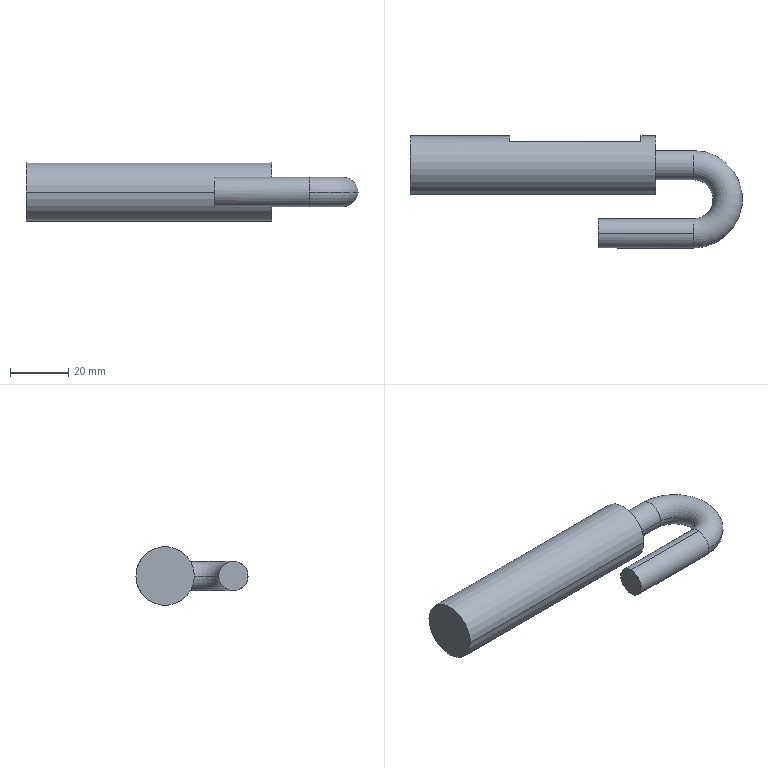Part | SolidWorks | features ICE 1, Revolution 1, Sweep 1 | 1 solid | 14 faces | box 113.683 x 38.367 x 20 mm | volume 32123 mm3 | cylinder 6 | plane 6 | torus 2 | commonest cylinder face diameters 10 x4 20 x2
STEP:
#1=CARTESIAN_POINT('',(55.,5.,0.));
#2=VERTEX_POINT('',#1);
#3=CARTESIAN_POINT('',(55.,-5.,0.));
#4=VERTEX_POINT('',#3);
#5=CARTESIAN_POINT('',(55.,0.,0.));
#6=DIRECTION('',(-1.,0.,0.));
#7=DIRECTION('',(0.,0.,-1.));
#8=AXIS2_PLACEMENT_3D('',#5,#6,#7);
#9=CIRCLE('',#8,5.);
#10=EDGE_CURVE('',#2,#4,#9,.T.);
#11=ORIENTED_EDGE('',*,*,#10,.F.);
#12=CARTESIAN_POINT('',(55.,-28.367,0.));
#13=VERTEX_POINT('',#12);
#14=CARTESIAN_POINT('',(55.,-11.683,0.));
#15=DIRECTION('',(0.,0.,-1.));
#16=DIRECTION('',(-1.,0.,0.));
#17=AXIS2_PLACEMENT_3D('',#14,#15,#16);
#18=CIRCLE('',#17,16.683);
#19=EDGE_CURVE('',#2,#13,#18,.T.);
#20=ORIENTED_EDGE('',*,*,#19,.T.);
#21=CARTESIAN_POINT('',(55.,-23.367,-5.));
#22=VERTEX_POINT('',#21);
#23=CARTESIAN_POINT('',(55.,-23.367,0.));
#24=DIRECTION('',(1.,0.,0.));
#25=DIRECTION('',(0.,0.,-1.));
#26=AXIS2_PLACEMENT_3D('',#23,#24,#25);
#27=CIRCLE('',#26,5.);
#28=EDGE_CURVE('',#13,#22,#27,.T.);
#29=ORIENTED_EDGE('',*,*,#28,.T.);
#30=CARTESIAN_POINT('',(55.,-18.367,0.));
#31=VERTEX_POINT('',#30);
#32=CARTESIAN_POINT('',(55.,-23.367,0.));
#33=DIRECTION('',(1.,0.,0.));
#34=DIRECTION('',(0.,0.,-1.));
#35=AXIS2_PLACEMENT_3D('',#32,#33,#34);
#36=CIRCLE('',#35,5.);
#37=EDGE_CURVE('',#22,#31,#36,.T.);
#38=ORIENTED_EDGE('',*,*,#37,.T.);
#39=CARTESIAN_POINT('',(55.,-11.683,0.));
#40=DIRECTION('',(0.,0.,-1.));
#41=DIRECTION('',(-1.,0.,0.));
#42=AXIS2_PLACEMENT_3D('',#39,#40,#41);
#43=CIRCLE('',#42,6.683);
#44=EDGE_CURVE('',#4,#31,#43,.T.);
#45=ORIENTED_EDGE('',*,*,#44,.F.);
#46=EDGE_LOOP('',(#11,#20,#29,#38,#45));
#47=FACE_OUTER_BOUND('',#46,.T.);
#48=CARTESIAN_POINT('',(55.,-11.683,0.));
#49=DIRECTION('',(0.,0.,-1.));
#50=DIRECTION('',(-1.,0.,0.));
#51=AXIS2_PLACEMENT_3D('',#48,#49,#50);
#52=TOROIDAL_SURFACE('',#51,11.683,5.);
#53=ADVANCED_FACE('',(#47),#52,.T.);
#54=ORIENTED_EDGE('',*,*,#37,.F.);
#55=CARTESIAN_POINT('',(22.334,-23.367,-5.));
#56=VERTEX_POINT('',#55);
#57=CARTESIAN_POINT('',(55.,-23.367,-5.));
#58=DIRECTION('',(-1.,0.,0.));
#59=VECTOR('',#58,1000.);
#60=LINE('',#57,#59);
#61=EDGE_CURVE('',#22,#56,#60,.T.);
#62=ORIENTED_EDGE('',*,*,#61,.T.);
#63=CARTESIAN_POINT('',(22.334,-23.367,5.));
#64=VERTEX_POINT('',#63);
#65=CARTESIAN_POINT('',(22.334,-23.367,0.));
#66=DIRECTION('',(1.,0.,0.));
#67=DIRECTION('',(0.,0.,-1.));
#68=AXIS2_PLACEMENT_3D('',#65,#66,#67);
#69=CIRCLE('',#68,5.);
#70=EDGE_CURVE('',#56,#64,#69,.T.);
#71=ORIENTED_EDGE('',*,*,#70,.T.);
#72=CARTESIAN_POINT('',(55.,-23.367,5.));
#73=VERTEX_POINT('',#72);
#74=CARTESIAN_POINT('',(55.,-23.367,5.));
#75=DIRECTION('',(-1.,0.,0.));
#76=VECTOR('',#75,1000.);
#77=LINE('',#74,#76);
#78=EDGE_CURVE('',#73,#64,#77,.T.);
#79=ORIENTED_EDGE('',*,*,#78,.F.);
#80=CARTESIAN_POINT('',(55.,-23.367,0.));
#81=DIRECTION('',(1.,0.,0.));
#82=DIRECTION('',(0.,0.,-1.));
#83=AXIS2_PLACEMENT_3D('',#80,#81,#82);
#84=CIRCLE('',#83,5.);
#85=EDGE_CURVE('',#31,#73,#84,.T.);
#86=ORIENTED_EDGE('',*,*,#85,.F.);
#87=EDGE_LOOP('',(#54,#62,#71,#79,#86));
#88=FACE_OUTER_BOUND('',#87,.T.);
#89=CARTESIAN_POINT('',(55.,-23.367,0.));
#90=DIRECTION('',(-1.,0.,0.));
#91=DIRECTION('',(0.,0.,1.));
#92=AXIS2_PLACEMENT_3D('',#89,#90,#91);
#93=CYLINDRICAL_SURFACE('',#92,5.);
#94=ADVANCED_FACE('',(#88),#93,.T.);
#95=CARTESIAN_POINT('',(42.,-5.,0.));
#96=VERTEX_POINT('',#95);
#97=CARTESIAN_POINT('',(42.,5.,0.));
#98=VERTEX_POINT('',#97);
#99=CARTESIAN_POINT('',(42.,0.,0.));
#100=DIRECTION('',(-1.,0.,0.));
#101=DIRECTION('',(0.,0.,-1.));
#102=AXIS2_PLACEMENT_3D('',#99,#100,#101);
#103=CIRCLE('',#102,5.);
#104=EDGE_CURVE('',#96,#98,#103,.T.);
#105=ORIENTED_EDGE('',*,*,#104,.F.);
#106=CARTESIAN_POINT('',(42.,-5.,0.));
#107=DIRECTION('',(1.,0.,0.));
#108=VECTOR('',#107,1000.);
#109=LINE('',#106,#108);
#110=EDGE_CURVE('',#96,#4,#109,.T.);
#111=ORIENTED_EDGE('',*,*,#110,.T.);
#112=CARTESIAN_POINT('',(55.,0.,0.));
#113=DIRECTION('',(-1.,0.,0.));
#114=DIRECTION('',(0.,0.,-1.));
#115=AXIS2_PLACEMENT_3D('',#112,#113,#114);
#116=CIRCLE('',#115,5.);
#117=EDGE_CURVE('',#4,#2,#116,.T.);
#118=ORIENTED_EDGE('',*,*,#117,.T.);
#119=CARTESIAN_POINT('',(42.,5.,0.));
#120=DIRECTION('',(1.,0.,0.));
#121=VECTOR('',#120,1000.);
#122=LINE('',#119,#121);
#123=EDGE_CURVE('',#98,#2,#122,.T.);
#124=ORIENTED_EDGE('',*,*,#123,.F.);
#125=EDGE_LOOP('',(#105,#111,#118,#124));
#126=FACE_OUTER_BOUND('',#125,.T.);
#127=CARTESIAN_POINT('',(42.,0.,0.));
#128=DIRECTION('',(1.,0.,0.));
#129=DIRECTION('',(0.,1.,0.));
#130=AXIS2_PLACEMENT_3D('',#127,#128,#129);
#131=CYLINDRICAL_SURFACE('',#130,5.);
#132=ADVANCED_FACE('',(#126),#131,.T.);
#133=CARTESIAN_POINT('',(42.,-10.,0.));
#134=VERTEX_POINT('',#133);
#135=CARTESIAN_POINT('',(42.,10.,0.));
#136=VERTEX_POINT('',#135);
#137=CARTESIAN_POINT('',(42.,0.,0.));
#138=DIRECTION('',(-1.,0.,0.));
#139=DIRECTION('',(0.,-1.,0.));
#140=AXIS2_PLACEMENT_3D('',#137,#138,#139);
#141=CIRCLE('',#140,10.);
#142=EDGE_CURVE('',#134,#136,#141,.T.);
#143=ORIENTED_EDGE('',*,*,#142,.T.);
#144=CARTESIAN_POINT('',(37.,10.,0.));
#145=VERTEX_POINT('',#144);
#146=CARTESIAN_POINT('',(-42.,10.,0.));
#147=DIRECTION('',(-1.,0.,0.));
#148=VECTOR('',#147,1000.);
#149=LINE('',#146,#148);
#150=EDGE_CURVE('',#136,#145,#149,.T.);
#151=ORIENTED_EDGE('',*,*,#150,.T.);
#152=CARTESIAN_POINT('',(37.,8.,6.));
#153=VERTEX_POINT('',#152);
#154=CARTESIAN_POINT('',(37.,0.,0.));
#155=DIRECTION('',(1.,0.,0.));
#156=DIRECTION('',(0.,1.,0.));
#157=AXIS2_PLACEMENT_3D('',#154,#155,#156);
#158=CIRCLE('',#157,10.);
#159=EDGE_CURVE('',#145,#153,#158,.T.);
#160=ORIENTED_EDGE('',*,*,#159,.T.);
#161=CARTESIAN_POINT('',(-8.,8.,6.));
#162=VERTEX_POINT('',#161);
#163=CARTESIAN_POINT('',(-42.,8.,6.));
#164=DIRECTION('',(1.,0.,0.));
#165=VECTOR('',#164,1000.);
#166=LINE('',#163,#165);
#167=EDGE_CURVE('',#162,#153,#166,.T.);
#168=ORIENTED_EDGE('',*,*,#167,.F.);
#169=CARTESIAN_POINT('',(-8.,10.,0.));
#170=VERTEX_POINT('',#169);
#171=CARTESIAN_POINT('',(-8.,0.,0.));
#172=DIRECTION('',(-1.,0.,0.));
#173=DIRECTION('',(0.,-1.,0.));
#174=AXIS2_PLACEMENT_3D('',#171,#172,#173);
#175=CIRCLE('',#174,10.);
#176=EDGE_CURVE('',#162,#170,#175,.T.);
#177=ORIENTED_EDGE('',*,*,#176,.T.);
#178=CARTESIAN_POINT('',(-42.,10.,0.));
#179=VERTEX_POINT('',#178);
#180=CARTESIAN_POINT('',(-42.,10.,0.));
#181=DIRECTION('',(-1.,0.,0.));
#182=VECTOR('',#181,1000.);
#183=LINE('',#180,#182);
#184=EDGE_CURVE('',#170,#179,#183,.T.);
#185=ORIENTED_EDGE('',*,*,#184,.T.);
#186=CARTESIAN_POINT('',(-42.,-10.,0.));
#187=VERTEX_POINT('',#186);
#188=CARTESIAN_POINT('',(-42.,0.,0.));
#189=DIRECTION('',(-1.,0.,0.));
#190=DIRECTION('',(0.,-1.,0.));
#191=AXIS2_PLACEMENT_3D('',#188,#189,#190);
#192=CIRCLE('',#191,10.);
#193=EDGE_CURVE('',#187,#179,#192,.T.);
#194=ORIENTED_EDGE('',*,*,#193,.F.);
#195=CARTESIAN_POINT('',(-42.,-10.,0.));
#196=DIRECTION('',(-1.,0.,0.));
#197=VECTOR('',#196,1000.);
#198=LINE('',#195,#197);
#199=EDGE_CURVE('',#134,#187,#198,.T.);
#200=ORIENTED_EDGE('',*,*,#199,.F.);
#201=EDGE_LOOP('',(#143,#151,#160,#168,#177,#185,#194,#200));
#202=FACE_OUTER_BOUND('',#201,.T.);
#203=CARTESIAN_POINT('',(-42.,0.,0.));
#204=DIRECTION('',(-1.,0.,0.));
#205=DIRECTION('',(0.,-1.,0.));
#206=AXIS2_PLACEMENT_3D('',#203,#204,#205);
#207=CYLINDRICAL_SURFACE('',#206,10.);
#208=ADVANCED_FACE('',(#202),#207,.T.);
#209=ORIENTED_EDGE('',*,*,#150,.F.);
#210=CARTESIAN_POINT('',(42.,0.,0.));
#211=DIRECTION('',(-1.,0.,0.));
#212=DIRECTION('',(0.,-1.,0.));
#213=AXIS2_PLACEMENT_3D('',#210,#211,#212);
#214=CIRCLE('',#213,10.);
#215=EDGE_CURVE('',#136,#134,#214,.T.);
#216=ORIENTED_EDGE('',*,*,#215,.T.);
#217=ORIENTED_EDGE('',*,*,#199,.T.);
#218=CARTESIAN_POINT('',(-42.,0.,0.));
#219=DIRECTION('',(-1.,0.,0.));
#220=DIRECTION('',(0.,-1.,0.));
#221=AXIS2_PLACEMENT_3D('',#218,#219,#220);
#222=CIRCLE('',#221,10.);
#223=EDGE_CURVE('',#179,#187,#222,.T.);
#224=ORIENTED_EDGE('',*,*,#223,.F.);
#225=ORIENTED_EDGE('',*,*,#184,.F.);
#226=CARTESIAN_POINT('',(-8.,8.,-6.));
#227=VERTEX_POINT('',#226);
#228=CARTESIAN_POINT('',(-8.,0.,0.));
#229=DIRECTION('',(-1.,0.,0.));
#230=DIRECTION('',(0.,-1.,0.));
#231=AXIS2_PLACEMENT_3D('',#228,#229,#230);
#232=CIRCLE('',#231,10.);
#233=EDGE_CURVE('',#170,#227,#232,.T.);
#234=ORIENTED_EDGE('',*,*,#233,.T.);
#235=CARTESIAN_POINT('',(37.,8.,-6.));
#236=VERTEX_POINT('',#235);
#237=CARTESIAN_POINT('',(-42.,8.,-6.));
#238=DIRECTION('',(-1.,0.,0.));
#239=VECTOR('',#238,1000.);
#240=LINE('',#237,#239);
#241=EDGE_CURVE('',#236,#227,#240,.T.);
#242=ORIENTED_EDGE('',*,*,#241,.F.);
#243=CARTESIAN_POINT('',(37.,0.,0.));
#244=DIRECTION('',(1.,0.,0.));
#245=DIRECTION('',(0.,1.,0.));
#246=AXIS2_PLACEMENT_3D('',#243,#244,#245);
#247=CIRCLE('',#246,10.);
#248=EDGE_CURVE('',#236,#145,#247,.T.);
#249=ORIENTED_EDGE('',*,*,#248,.T.);
#250=EDGE_LOOP('',(#209,#216,#217,#224,#225,#234,#242,#249));
#251=FACE_OUTER_BOUND('',#250,.T.);
#252=CARTESIAN_POINT('',(-42.,0.,0.));
#253=DIRECTION('',(-1.,0.,0.));
#254=DIRECTION('',(0.,-1.,0.));
#255=AXIS2_PLACEMENT_3D('',#252,#253,#254);
#256=CYLINDRICAL_SURFACE('',#255,10.);
#257=ADVANCED_FACE('',(#251),#256,.T.);
#258=ORIENTED_EDGE('',*,*,#193,.T.);
#259=ORIENTED_EDGE('',*,*,#223,.T.);
#260=EDGE_LOOP('',(#258,#259));
#261=FACE_OUTER_BOUND('',#260,.T.);
#262=CARTESIAN_POINT('',(-42.,0.,0.));
#263=DIRECTION('',(1.,0.,0.));
#264=DIRECTION('',(0.,1.,0.));
#265=AXIS2_PLACEMENT_3D('',#262,#263,#264);
#266=PLANE('',#265);
#267=ADVANCED_FACE('',(#261),#266,.F.);
#268=CARTESIAN_POINT('',(42.,0.,0.));
#269=DIRECTION('',(-1.,0.,0.));
#270=DIRECTION('',(0.,0.,-1.));
#271=AXIS2_PLACEMENT_3D('',#268,#269,#270);
#272=CIRCLE('',#271,5.);
#273=EDGE_CURVE('',#98,#96,#272,.T.);
#274=ORIENTED_EDGE('',*,*,#273,.T.);
#275=ORIENTED_EDGE('',*,*,#104,.T.);
#276=EDGE_LOOP('',(#274,#275));
#277=FACE_BOUND('',#276,.T.);
#278=ORIENTED_EDGE('',*,*,#142,.F.);
#279=ORIENTED_EDGE('',*,*,#215,.F.);
#280=EDGE_LOOP('',(#278,#279));
#281=FACE_OUTER_BOUND('',#280,.T.);
#282=CARTESIAN_POINT('',(42.,0.,0.));
#283=DIRECTION('',(-1.,0.,0.));
#284=DIRECTION('',(0.,-1.,0.));
#285=AXIS2_PLACEMENT_3D('',#282,#283,#284);
#286=PLANE('',#285);
#287=ADVANCED_FACE('',(#277,#281),#286,.F.);
#288=CARTESIAN_POINT('',(-8.,8.,-17.202));
#289=DIRECTION('',(0.,0.,1.));
#290=VECTOR('',#289,1000.);
#291=LINE('',#288,#290);
#292=EDGE_CURVE('',#227,#162,#291,.T.);
#293=ORIENTED_EDGE('',*,*,#292,.F.);
#294=ORIENTED_EDGE('',*,*,#233,.F.);
#295=ORIENTED_EDGE('',*,*,#176,.F.);
#296=EDGE_LOOP('',(#293,#294,#295));
#297=FACE_OUTER_BOUND('',#296,.T.);
#298=CARTESIAN_POINT('',(-8.,8.,-17.202));
#299=DIRECTION('',(-1.,0.,0.));
#300=DIRECTION('',(0.,-1.,0.));
#301=AXIS2_PLACEMENT_3D('',#298,#299,#300);
#302=PLANE('',#301);
#303=ADVANCED_FACE('',(#297),#302,.F.);
#304=ORIENTED_EDGE('',*,*,#248,.F.);
#305=CARTESIAN_POINT('',(37.,8.,-17.202));
#306=DIRECTION('',(0.,0.,-1.));
#307=VECTOR('',#306,1000.);
#308=LINE('',#305,#307);
#309=EDGE_CURVE('',#153,#236,#308,.T.);
#310=ORIENTED_EDGE('',*,*,#309,.F.);
#311=ORIENTED_EDGE('',*,*,#159,.F.);
#312=EDGE_LOOP('',(#304,#310,#311));
#313=FACE_OUTER_BOUND('',#312,.T.);
#314=CARTESIAN_POINT('',(37.,8.,-17.202));
#315=DIRECTION('',(1.,0.,0.));
#316=DIRECTION('',(0.,1.,0.));
#317=AXIS2_PLACEMENT_3D('',#314,#315,#316);
#318=PLANE('',#317);
#319=ADVANCED_FACE('',(#313),#318,.F.);
#320=ORIENTED_EDGE('',*,*,#241,.T.);
#321=ORIENTED_EDGE('',*,*,#292,.T.);
#322=ORIENTED_EDGE('',*,*,#167,.T.);
#323=ORIENTED_EDGE('',*,*,#309,.T.);
#324=EDGE_LOOP('',(#320,#321,#322,#323));
#325=FACE_OUTER_BOUND('',#324,.T.);
#326=CARTESIAN_POINT('',(0.,8.,0.));
#327=DIRECTION('',(0.,1.,0.));
#328=DIRECTION('',(-1.,0.,0.));
#329=AXIS2_PLACEMENT_3D('',#326,#327,#328);
#330=PLANE('',#329);
#331=ADVANCED_FACE('',(#325),#330,.T.);
#332=ORIENTED_EDGE('',*,*,#61,.F.);
#333=ORIENTED_EDGE('',*,*,#28,.F.);
#334=CARTESIAN_POINT('',(55.,-23.367,0.));
#335=DIRECTION('',(1.,0.,0.));
#336=DIRECTION('',(0.,0.,-1.));
#337=AXIS2_PLACEMENT_3D('',#334,#335,#336);
#338=CIRCLE('',#337,5.);
#339=EDGE_CURVE('',#73,#13,#338,.T.);
#340=ORIENTED_EDGE('',*,*,#339,.F.);
#341=ORIENTED_EDGE('',*,*,#78,.T.);
#342=CARTESIAN_POINT('',(22.334,-23.367,0.));
#343=DIRECTION('',(1.,0.,0.));
#344=DIRECTION('',(0.,0.,-1.));
#345=AXIS2_PLACEMENT_3D('',#342,#343,#344);
#346=CIRCLE('',#345,5.);
#347=EDGE_CURVE('',#64,#56,#346,.T.);
#348=ORIENTED_EDGE('',*,*,#347,.T.);
#349=EDGE_LOOP('',(#332,#333,#340,#341,#348));
#350=FACE_OUTER_BOUND('',#349,.T.);
#351=CARTESIAN_POINT('',(55.,-23.367,0.));
#352=DIRECTION('',(-1.,0.,0.));
#353=DIRECTION('',(0.,0.,1.));
#354=AXIS2_PLACEMENT_3D('',#351,#352,#353);
#355=CYLINDRICAL_SURFACE('',#354,5.);
#356=ADVANCED_FACE('',(#350),#355,.T.);
#357=ORIENTED_EDGE('',*,*,#19,.F.);
#358=ORIENTED_EDGE('',*,*,#117,.F.);
#359=ORIENTED_EDGE('',*,*,#44,.T.);
#360=ORIENTED_EDGE('',*,*,#85,.T.);
#361=ORIENTED_EDGE('',*,*,#339,.T.);
#362=EDGE_LOOP('',(#357,#358,#359,#360,#361));
#363=FACE_OUTER_BOUND('',#362,.T.);
#364=CARTESIAN_POINT('',(55.,-11.683,0.));
#365=DIRECTION('',(0.,0.,-1.));
#366=DIRECTION('',(-1.,0.,0.));
#367=AXIS2_PLACEMENT_3D('',#364,#365,#366);
#368=TOROIDAL_SURFACE('',#367,11.683,5.);
#369=ADVANCED_FACE('',(#363),#368,.T.);
#370=ORIENTED_EDGE('',*,*,#110,.F.);
#371=ORIENTED_EDGE('',*,*,#273,.F.);
#372=ORIENTED_EDGE('',*,*,#123,.T.);
#373=ORIENTED_EDGE('',*,*,#10,.T.);
#374=EDGE_LOOP('',(#370,#371,#372,#373));
#375=FACE_OUTER_BOUND('',#374,.T.);
#376=CARTESIAN_POINT('',(42.,0.,0.));
#377=DIRECTION('',(1.,0.,0.));
#378=DIRECTION('',(0.,1.,0.));
#379=AXIS2_PLACEMENT_3D('',#376,#377,#378);
#380=CYLINDRICAL_SURFACE('',#379,5.);
#381=ADVANCED_FACE('',(#375),#380,.T.);
#382=ORIENTED_EDGE('',*,*,#347,.F.);
#383=ORIENTED_EDGE('',*,*,#70,.F.);
#384=EDGE_LOOP('',(#382,#383));
#385=FACE_OUTER_BOUND('',#384,.T.);
#386=CARTESIAN_POINT('',(22.334,-23.367,0.));
#387=DIRECTION('',(1.,0.,0.));
#388=DIRECTION('',(0.,0.,-1.));
#389=AXIS2_PLACEMENT_3D('',#386,#387,#388);
#390=PLANE('',#389);
#391=ADVANCED_FACE('',(#385),#390,.F.);
#392=CLOSED_SHELL('',(#53,#94,#132,#208,#257,#267,#287,#303,#319,#331,#356,#369,#381,#391));
#393=MANIFOLD_SOLID_BREP('',#392);
#394=CARTESIAN_POINT('',(0.,0.,0.));
#395=DIRECTION('',(0.,0.,1.));
#396=DIRECTION('',(1.,0.,0.));
#397=AXIS2_PLACEMENT_3D('',#394,#395,#396);
#398=(LENGTH_UNIT()NAMED_UNIT(*)SI_UNIT(.MILLI.,.METRE.));
#399=UNCERTAINTY_MEASURE_WITH_UNIT(LENGTH_MEASURE(0.00001),#398,'','');
#400=(NAMED_UNIT(*)PLANE_ANGLE_UNIT()SI_UNIT($,.RADIAN.));
#401=(NAMED_UNIT(*)SI_UNIT($,.STERADIAN.)SOLID_ANGLE_UNIT());
#402=(GEOMETRIC_REPRESENTATION_CONTEXT(3)GLOBAL_UNCERTAINTY_ASSIGNED_CONTEXT((#399))GLOBAL_UNIT_ASSIGNED_CONTEXT((#398,#400,#401))REPRESENTATION_CONTEXT('',''));
#403=ADVANCED_BREP_SHAPE_REPRESENTATION('',(#393,#397),#402);